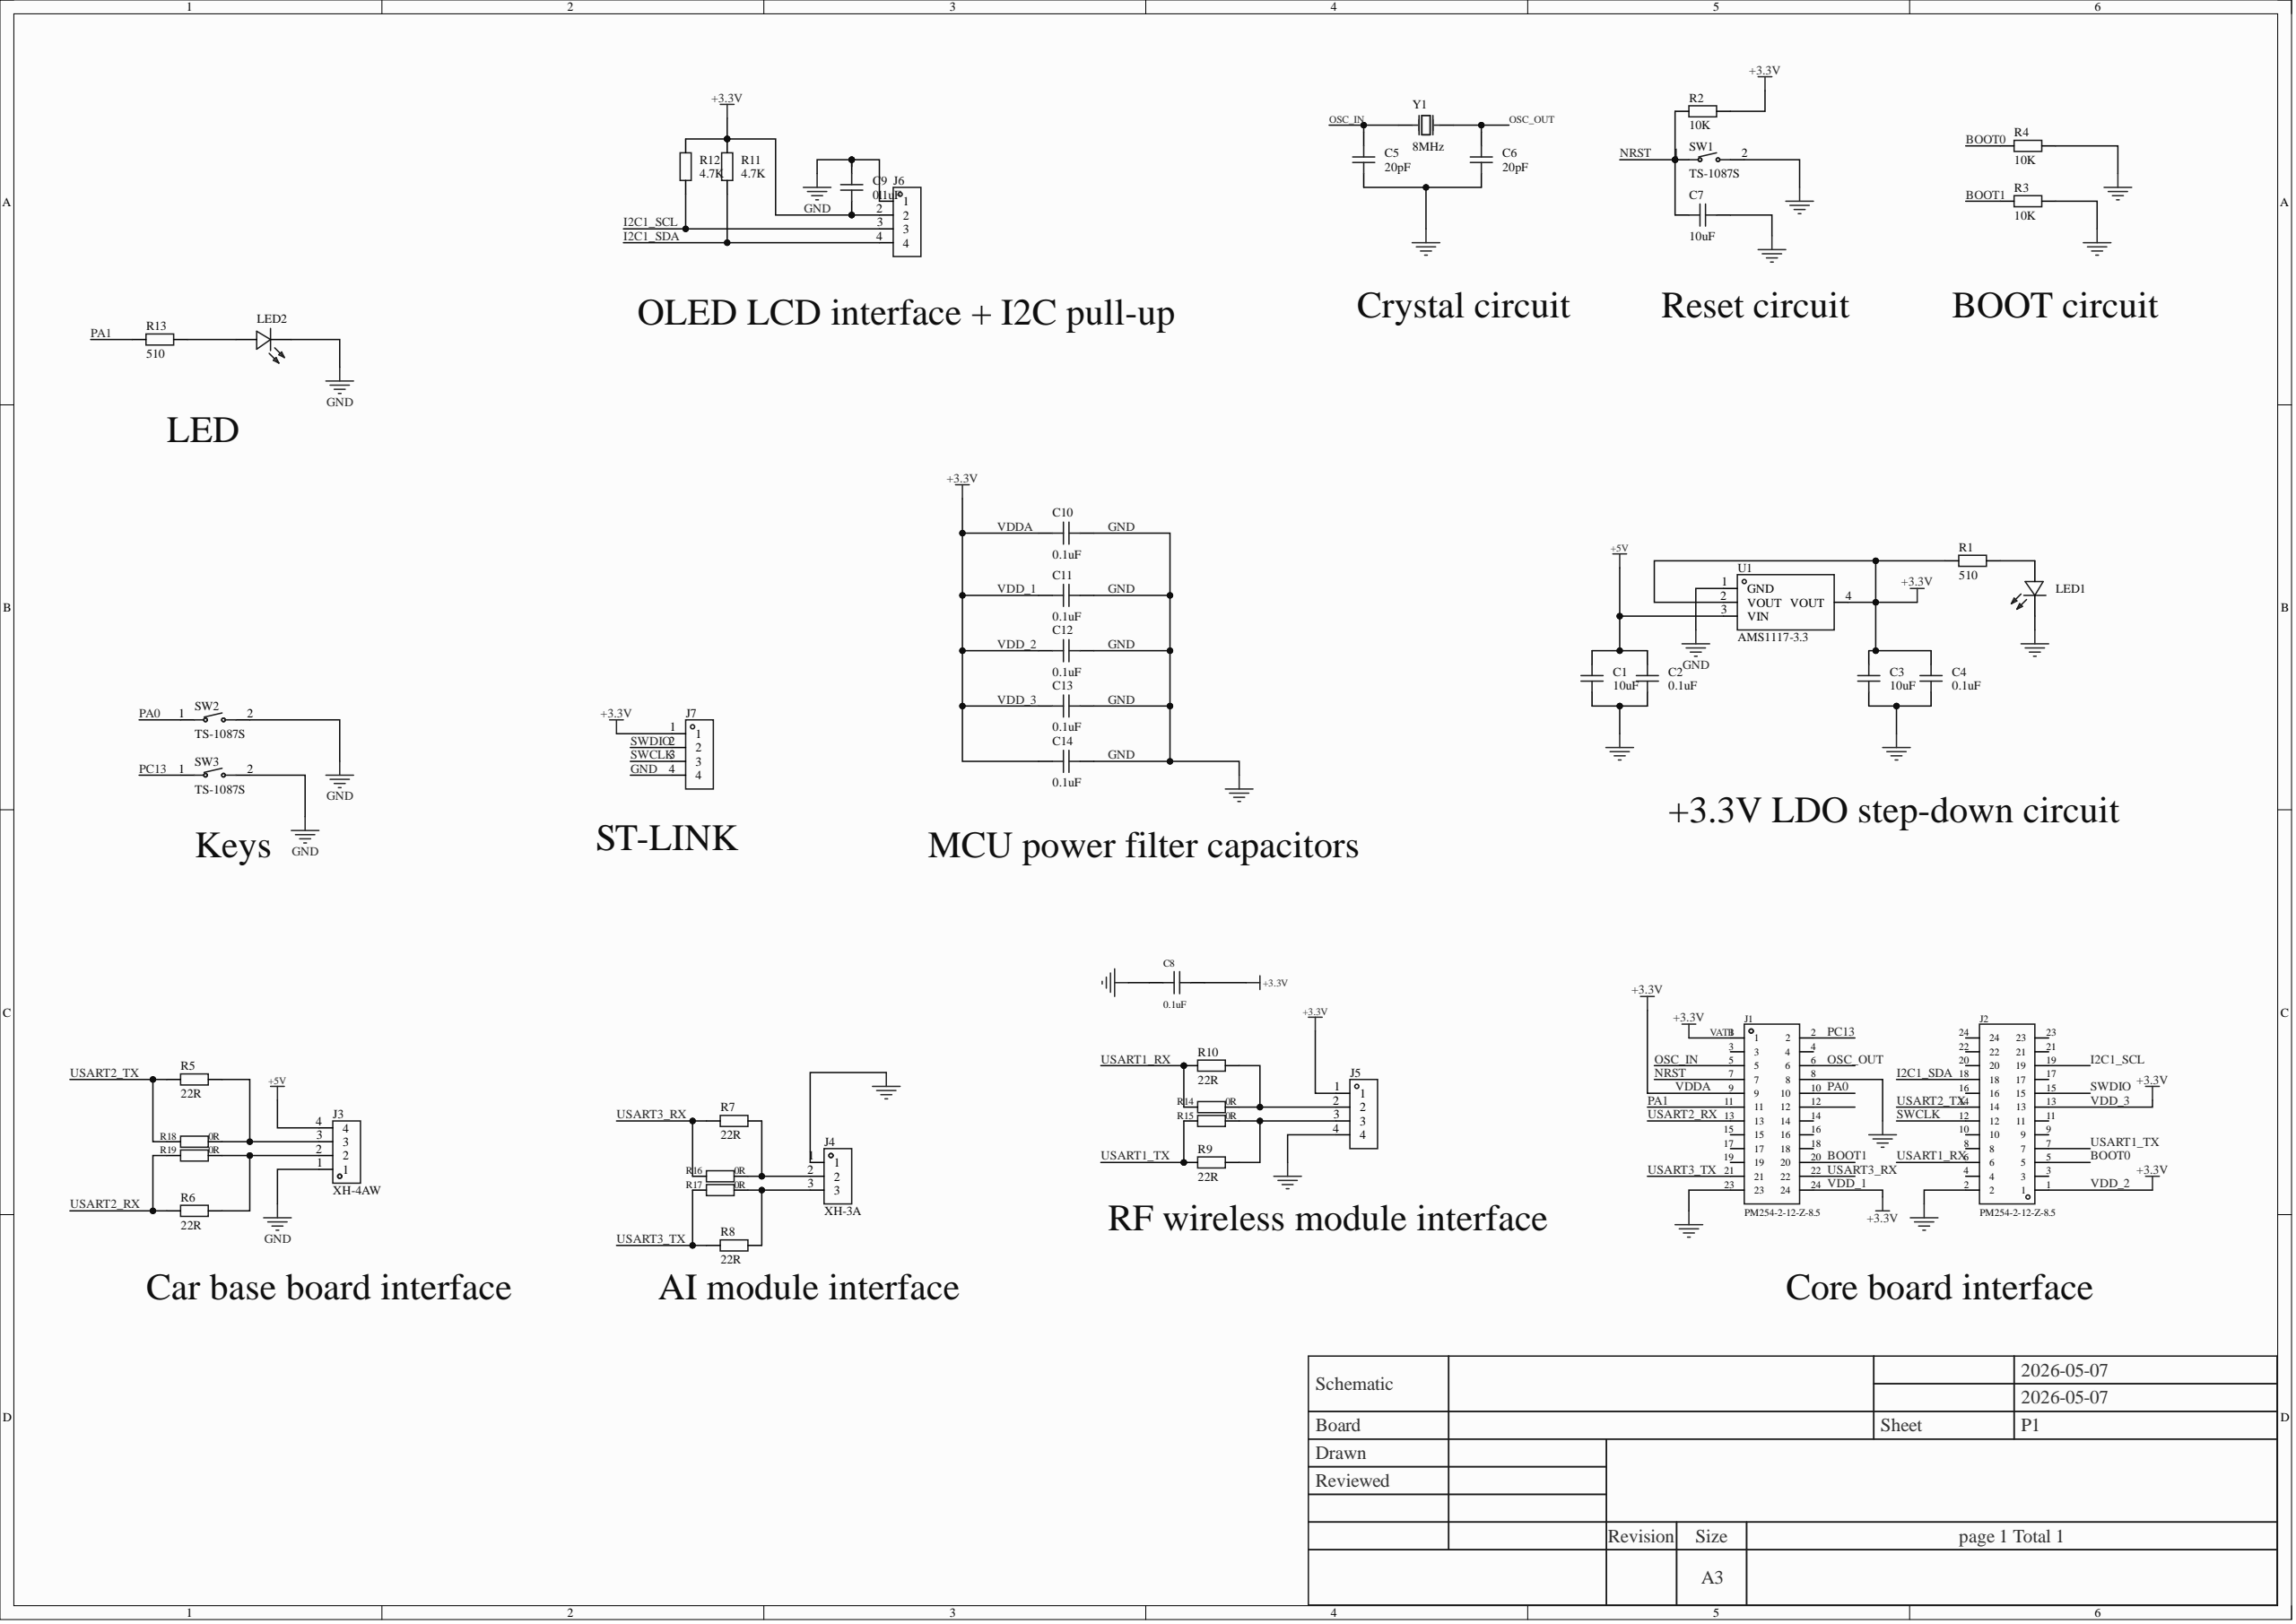Circuit board | Altium Designer | 47 parts | 29 nets
Bill of materials:
Comment,Description,Designator,Footprint,LibRef,Quantity
"10uF","","C1, C3, C7","C0805","CAP_0603","3"
"0.1uF","","C2, C4, C9, C10, C11, C12, C13, C14","C0805","CAP_0603","8"
"20pF","","C5, C6","C0805","CAP_0603","2"
"0.1uF","","C8","C0603","CAP_0603","1"
"PM254-2-12-Z-8.5","","J1, J2","HDR-TH_24P-P2.54-V-F-R2-C12-S2.54-2","PM254-2-12-Z-8.5","2"
"XH-4AW","","J3","CONN-TH_XH-4AW","XH-4AW","1"
"XH-3A","","J4","CONN-TH_XH-3A","XH-3A","1"
"","","J5, J6, J7","CONN-TH_4P-P2.54-L10.2-W2.5","POGOPIN-4P-2.54-17.0H-2.0T","3"
"KT-0805W","","LED1","LED0805-R-RD","KT-0805W","1"
"","","LED2","LED0805-R-RD","KT-0805W","1"
"510","","R1, R13","R0805","Res_0603","2"
"10K","","R2, R3, R4","R0805","Res_0603","3"
"22R","","R5, R6, R7, R8, R9, R10","R0805","Res_0603","6"
"4.7K","","R11, R12","R0805","Res_0603","2"
"0R","","R14, R15, R16, R17, R18, R19","R0603","Res_0603","6"
"TS-1087S","","SW1, SW2, SW3","SW-SMD_L5.2-W5.2-P3.70-LS6.4","TS-1087S-04026","3"
"AMS1117-3.3","","U1","SOT-223-3_L6.5-W3.4-P2.30-LS7.0-BR","AMS1117-3.3_C6186","1"
"8MHz","","Y1","CRYSTAL-SMD_L11.5-W4.8-LS12.7","X49SM8MSD2SC","1"
Netlist (Protel format):
[
C1
C0805
10uF



]
[
C2
C0805
0.1uF



]
[
C3
C0805
10uF



]
[
C4
C0805
0.1uF



]
[
C5
C0805
20pF



]
[
C6
C0805
20pF



]
[
C7
C0805
10uF



]
[
C8
C0603
0.1uF



]
[
C9
C0805
0.1uF



]
[
C10
C0805
0.1uF



]
[
C11
C0805
0.1uF



]
[
C12
C0805
0.1uF



]
[
C13
C0805
0.1uF



]
[
C14
C0805
0.1uF



]
[
J1
HDR-TH_24P-P2.54-V-F-R2-C12-S2.54-2
PM254-2-12-Z-8.5



]
[
J2
HDR-TH_24P-P2.54-V-F-R2-C12-S2.54-2
PM254-2-12-Z-8.5



]
[
J3
CONN-TH_XH-4AW
XH-4AW



]
[
J4
CONN-TH_XH-3A
XH-3A



]
[
J5
CONN-TH_4P-P2.54-L10.2-W2.5




]
[
J6
CONN-TH_4P-P2.54-L10.2-W2.5




]
[
J7
CONN-TH_4P-P2.54-L10.2-W2.5




]
[
LED1
LED0805-R-RD
KT-0805W



]
[
LED2
LED0805-R-RD




]
[
R1
R0805
510



]
[
R2
R0805
10K



]
[
R3
R0805
10K



]
[
R4
R0805
10K



]
[
R5
R0805
22R



]
[
R6
R0805
22R



]
[
R7
R0805
22R



]
[
R8
R0805
22R



]
[
R9
R0805
22R



]
[
R10
R0805
22R



]
[
R11
R0805
4.7K



]
[
R12
R0805
4.7K



]
[
R13
R0805
510



]
[
R14
R0603
0R



]
[
R15
R0603
0R



]
[
R16
R0603
0R



]
[
R17
R0603
0R



]
[
R18
R0603
0R



]
[
R19
R0603
0R



]
[
SW1
SW-SMD_L5.2-W5.2-P3.70-LS6.4
TS-1087S



]
[
SW2
SW-SMD_L5.2-W5.2-P3.70-LS6.4
TS-1087S



]
[
SW3
SW-SMD_L5.2-W5.2-P3.70-LS6.4
TS-1087S



]
[
U1
SOT-223-3_L6.5-W3.4-P2.30-LS7.0-BR
AMS1117-3.3



]
[
Y1
CRYSTAL-SMD_L11.5-W4.8-LS12.7
8MHz



]
(
VATB
C3-2
C4-2
C8-2
C9-1
C10-1
C11-1
C12-1
C13-1
C14-1
J1-1
J1-9
J1-24
J2-1
J2-13
J5-1
J6-2
J7-1
R1-1
R2-2
R11-2
R12-2
U1-2
U1-4
)
(
USART3_TX
J1-21
R8-1
R17-1
)
(
USART3_RX
J1-22
R7-1
R16-1
)
(
USART2_TX
J2-14
R5-1
R18-1
)
(
USART2_RX
J1-13
R6-1
R19-1
)
(
USART1_TX
J2-7
R9-1
R15-1
)
(
USART1_RX
J2-6
R10-1
R14-1
)
(
SWDIO
J2-15
J7-2
)
(
SWCLK
J2-12
J7-3
)
(
PC13
J1-2
SW3-1
)
(
PA1
J1-11
R13-1
)
(
PA0
J1-10
SW2-1
)
(
OSC_OUT
C6-2
J1-6
Y1-1
)
(
OSC_IN
C5-2
J1-5
Y1-2
)
(
NRST
C7-1
J1-7
R2-1
SW1-1
)
(
NetLED2_1
LED2-1
R13-2
)
(
NetLED1_1
LED1-1
R1-2
)
(
NetJ5_3
J5-3
R9-2
R15-2
)
(
NetJ5_2
J5-2
R10-2
R14-2
)
(
NetJ4_3
J4-3
R8-2
R17-2
)
(
NetJ4_2
J4-2
R7-2
R16-2
)
(
NetJ3_3
J3-3
R5-2
R18-2
)
(
NetJ3_2
J3-2
R6-2
R19-2
)
(
I2C1_SDA
J2-18
J6-4
R11-1
)
(
I2C1_SCL
J2-19
J6-3
R12-1
)
(
GND
C1-2
C2-2
C3-1
C4-1
C5-1
C6-1
C7-2
C8-1
C9-2
C10-2
C11-2
C12-2
C13-2
C14-2
J1-8
J1-23
J2-2
J3-1
J4-1
J5-4
J6-1
J7-4
LED1-2
LED2-2
R3-2
R4-2
SW1-2
SW2-2
SW3-2
U1-1
)
(
BOOT1
J1-20
R3-1
)
(
BOOT0
J2-5
R4-1
)
(
+5V
C1-1
C2-1
J3-4
U1-3
)